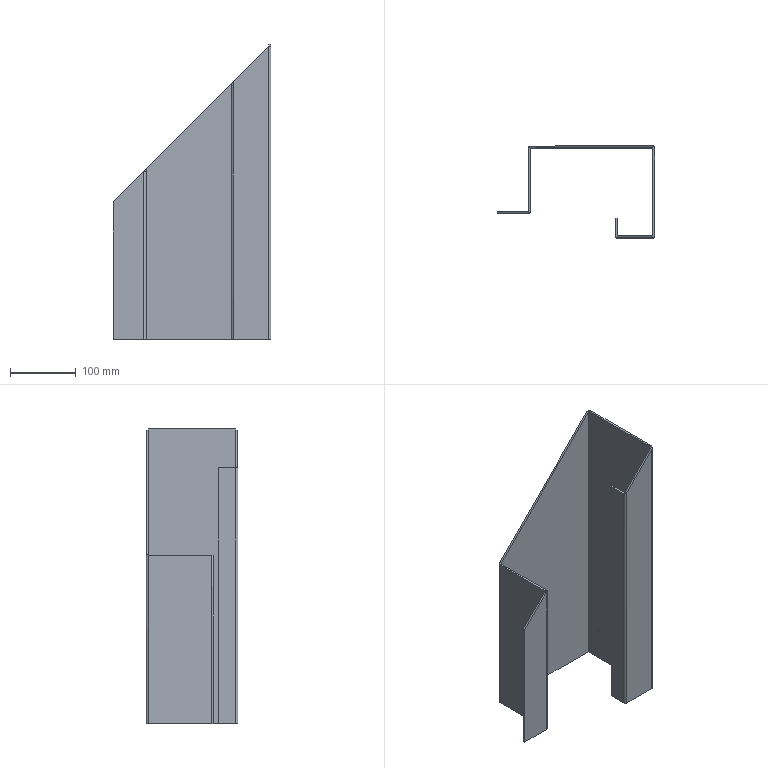Part | STEP file | SX-S32 | 1 solid | 52 faces | box 240 x 140 x 450 mm | volume 598692 mm3 | plane 33 | cylinder 14 | spline 5 | commonest cylinder face diameters 0.4 x5 6.4 x5 5 x4